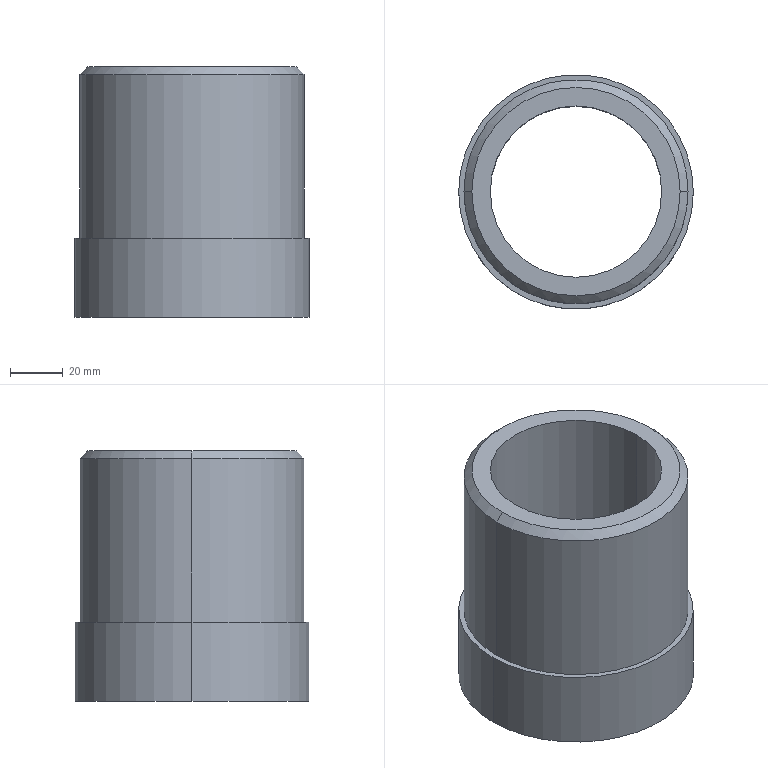Part | SolidWorks | features Chamfer 1, Extrusion 1, ICE 1 | 1 solid | 11 faces | box 89 x 89 x 95 mm | volume 239064 mm3 | cylinder 6 | plane 3 | cone 2 | commonest cylinder face diameters 65 x2 85 x2 89 x2
STEP:
#1=CARTESIAN_POINT('',(39.5,0.,95.));
#2=VERTEX_POINT('',#1);
#3=CARTESIAN_POINT('',(-39.5,0.,95.));
#4=VERTEX_POINT('',#3);
#5=CARTESIAN_POINT('',(0.,0.,95.));
#6=DIRECTION('',(0.,0.,1.));
#7=DIRECTION('',(1.,0.,0.));
#8=AXIS2_PLACEMENT_3D('',#5,#6,#7);
#9=CIRCLE('',#8,39.5);
#10=EDGE_CURVE('',#2,#4,#9,.T.);
#11=ORIENTED_EDGE('',*,*,#10,.F.);
#12=CARTESIAN_POINT('',(42.5,0.,92.));
#13=VERTEX_POINT('',#12);
#14=CARTESIAN_POINT('',(39.5,0.,95.));
#15=DIRECTION('',(0.7071,0.,-0.7071));
#16=VECTOR('',#15,1000.);
#17=LINE('',#14,#16);
#18=EDGE_CURVE('',#2,#13,#17,.T.);
#19=ORIENTED_EDGE('',*,*,#18,.T.);
#20=CARTESIAN_POINT('',(-42.5,0.,92.));
#21=VERTEX_POINT('',#20);
#22=CARTESIAN_POINT('',(0.,0.,92.));
#23=DIRECTION('',(0.,0.,-1.));
#24=DIRECTION('',(1.,0.,0.));
#25=AXIS2_PLACEMENT_3D('',#22,#23,#24);
#26=CIRCLE('',#25,42.5);
#27=EDGE_CURVE('',#21,#13,#26,.T.);
#28=ORIENTED_EDGE('',*,*,#27,.F.);
#29=CARTESIAN_POINT('',(-39.5,0.,95.));
#30=DIRECTION('',(-0.7071,0.,-0.7071));
#31=VECTOR('',#30,1000.);
#32=LINE('',#29,#31);
#33=EDGE_CURVE('',#4,#21,#32,.T.);
#34=ORIENTED_EDGE('',*,*,#33,.F.);
#35=EDGE_LOOP('',(#11,#19,#28,#34));
#36=FACE_OUTER_BOUND('',#35,.T.);
#37=CARTESIAN_POINT('',(0.,0.,95.));
#38=DIRECTION('',(0.,0.,-1.));
#39=DIRECTION('',(-1.,0.,0.));
#40=AXIS2_PLACEMENT_3D('',#37,#38,#39);
#41=CONICAL_SURFACE('',#40,39.5,0.7854);
#42=ADVANCED_FACE('',(#36),#41,.T.);
#43=CARTESIAN_POINT('',(42.5,0.,30.));
#44=VERTEX_POINT('',#43);
#45=CARTESIAN_POINT('',(-42.5,0.,30.));
#46=VERTEX_POINT('',#45);
#47=CARTESIAN_POINT('',(0.,0.,30.));
#48=DIRECTION('',(0.,0.,1.));
#49=DIRECTION('',(1.,0.,0.));
#50=AXIS2_PLACEMENT_3D('',#47,#48,#49);
#51=CIRCLE('',#50,42.5);
#52=EDGE_CURVE('',#44,#46,#51,.T.);
#53=ORIENTED_EDGE('',*,*,#52,.T.);
#54=CARTESIAN_POINT('',(-42.5,0.,30.));
#55=DIRECTION('',(0.,0.,1.));
#56=VECTOR('',#55,1000.);
#57=LINE('',#54,#56);
#58=EDGE_CURVE('',#46,#21,#57,.T.);
#59=ORIENTED_EDGE('',*,*,#58,.T.);
#60=ORIENTED_EDGE('',*,*,#27,.T.);
#61=CARTESIAN_POINT('',(42.5,0.,30.));
#62=DIRECTION('',(0.,0.,1.));
#63=VECTOR('',#62,1000.);
#64=LINE('',#61,#63);
#65=EDGE_CURVE('',#44,#13,#64,.T.);
#66=ORIENTED_EDGE('',*,*,#65,.F.);
#67=EDGE_LOOP('',(#53,#59,#60,#66));
#68=FACE_OUTER_BOUND('',#67,.T.);
#69=CARTESIAN_POINT('',(0.,0.,30.));
#70=DIRECTION('',(0.,0.,1.));
#71=DIRECTION('',(1.,0.,0.));
#72=AXIS2_PLACEMENT_3D('',#69,#70,#71);
#73=CYLINDRICAL_SURFACE('',#72,42.5);
#74=ADVANCED_FACE('',(#68),#73,.T.);
#75=CARTESIAN_POINT('',(-32.5,0.,95.));
#76=VERTEX_POINT('',#75);
#77=CARTESIAN_POINT('',(32.5,0.,95.));
#78=VERTEX_POINT('',#77);
#79=CARTESIAN_POINT('',(0.,0.,95.));
#80=DIRECTION('',(0.,0.,1.));
#81=DIRECTION('',(1.,0.,0.));
#82=AXIS2_PLACEMENT_3D('',#79,#80,#81);
#83=CIRCLE('',#82,32.5);
#84=EDGE_CURVE('',#76,#78,#83,.T.);
#85=ORIENTED_EDGE('',*,*,#84,.T.);
#86=CARTESIAN_POINT('',(32.5,0.,0.));
#87=VERTEX_POINT('',#86);
#88=CARTESIAN_POINT('',(32.5,0.,95.));
#89=DIRECTION('',(0.,0.,-1.));
#90=VECTOR('',#89,1000.);
#91=LINE('',#88,#90);
#92=EDGE_CURVE('',#78,#87,#91,.T.);
#93=ORIENTED_EDGE('',*,*,#92,.T.);
#94=CARTESIAN_POINT('',(-32.5,0.,0.));
#95=VERTEX_POINT('',#94);
#96=CARTESIAN_POINT('',(0.,0.,0.));
#97=DIRECTION('',(0.,0.,1.));
#98=DIRECTION('',(1.,0.,0.));
#99=AXIS2_PLACEMENT_3D('',#96,#97,#98);
#100=CIRCLE('',#99,32.5);
#101=EDGE_CURVE('',#95,#87,#100,.T.);
#102=ORIENTED_EDGE('',*,*,#101,.F.);
#103=CARTESIAN_POINT('',(-32.5,0.,95.));
#104=DIRECTION('',(0.,0.,-1.));
#105=VECTOR('',#104,1000.);
#106=LINE('',#103,#105);
#107=EDGE_CURVE('',#76,#95,#106,.T.);
#108=ORIENTED_EDGE('',*,*,#107,.F.);
#109=EDGE_LOOP('',(#85,#93,#102,#108));
#110=FACE_OUTER_BOUND('',#109,.T.);
#111=CARTESIAN_POINT('',(0.,0.,95.));
#112=DIRECTION('',(0.,0.,-1.));
#113=DIRECTION('',(-1.,0.,0.));
#114=AXIS2_PLACEMENT_3D('',#111,#112,#113);
#115=CYLINDRICAL_SURFACE('',#114,32.5);
#116=ADVANCED_FACE('',(#110),#115,.F.);
#117=CARTESIAN_POINT('',(44.5,0.,30.));
#118=VERTEX_POINT('',#117);
#119=CARTESIAN_POINT('',(-44.5,0.,30.));
#120=VERTEX_POINT('',#119);
#121=CARTESIAN_POINT('',(0.,0.,30.));
#122=DIRECTION('',(0.,0.,1.));
#123=DIRECTION('',(1.,0.,0.));
#124=AXIS2_PLACEMENT_3D('',#121,#122,#123);
#125=CIRCLE('',#124,44.5);
#126=EDGE_CURVE('',#118,#120,#125,.T.);
#127=ORIENTED_EDGE('',*,*,#126,.F.);
#128=CARTESIAN_POINT('',(44.5,0.,0.));
#129=VERTEX_POINT('',#128);
#130=CARTESIAN_POINT('',(44.5,0.,95.));
#131=DIRECTION('',(0.,0.,-1.));
#132=VECTOR('',#131,1000.);
#133=LINE('',#130,#132);
#134=EDGE_CURVE('',#118,#129,#133,.T.);
#135=ORIENTED_EDGE('',*,*,#134,.T.);
#136=CARTESIAN_POINT('',(-44.5,0.,0.));
#137=VERTEX_POINT('',#136);
#138=CARTESIAN_POINT('',(0.,0.,0.));
#139=DIRECTION('',(0.,0.,1.));
#140=DIRECTION('',(1.,0.,0.));
#141=AXIS2_PLACEMENT_3D('',#138,#139,#140);
#142=CIRCLE('',#141,44.5);
#143=EDGE_CURVE('',#129,#137,#142,.T.);
#144=ORIENTED_EDGE('',*,*,#143,.T.);
#145=CARTESIAN_POINT('',(-44.5,0.,95.));
#146=DIRECTION('',(0.,0.,-1.));
#147=VECTOR('',#146,1000.);
#148=LINE('',#145,#147);
#149=EDGE_CURVE('',#120,#137,#148,.T.);
#150=ORIENTED_EDGE('',*,*,#149,.F.);
#151=EDGE_LOOP('',(#127,#135,#144,#150));
#152=FACE_OUTER_BOUND('',#151,.T.);
#153=CARTESIAN_POINT('',(0.,0.,95.));
#154=DIRECTION('',(0.,0.,-1.));
#155=DIRECTION('',(-1.,0.,0.));
#156=AXIS2_PLACEMENT_3D('',#153,#154,#155);
#157=CYLINDRICAL_SURFACE('',#156,44.5);
#158=ADVANCED_FACE('',(#152),#157,.T.);
#159=CARTESIAN_POINT('',(0.,0.,95.));
#160=DIRECTION('',(0.,0.,1.));
#161=DIRECTION('',(1.,0.,0.));
#162=AXIS2_PLACEMENT_3D('',#159,#160,#161);
#163=CIRCLE('',#162,39.5);
#164=EDGE_CURVE('',#4,#2,#163,.T.);
#165=ORIENTED_EDGE('',*,*,#164,.T.);
#166=ORIENTED_EDGE('',*,*,#10,.T.);
#167=EDGE_LOOP('',(#165,#166));
#168=FACE_OUTER_BOUND('',#167,.T.);
#169=ORIENTED_EDGE('',*,*,#84,.F.);
#170=CARTESIAN_POINT('',(0.,0.,95.));
#171=DIRECTION('',(0.,0.,1.));
#172=DIRECTION('',(1.,0.,0.));
#173=AXIS2_PLACEMENT_3D('',#170,#171,#172);
#174=CIRCLE('',#173,32.5);
#175=EDGE_CURVE('',#78,#76,#174,.T.);
#176=ORIENTED_EDGE('',*,*,#175,.F.);
#177=EDGE_LOOP('',(#169,#176));
#178=FACE_BOUND('',#177,.T.);
#179=CARTESIAN_POINT('',(0.,0.,95.));
#180=DIRECTION('',(0.,0.,1.));
#181=DIRECTION('',(1.,0.,0.));
#182=AXIS2_PLACEMENT_3D('',#179,#180,#181);
#183=PLANE('',#182);
#184=ADVANCED_FACE('',(#168,#178),#183,.T.);
#185=ORIENTED_EDGE('',*,*,#134,.F.);
#186=CARTESIAN_POINT('',(0.,0.,30.));
#187=DIRECTION('',(0.,0.,1.));
#188=DIRECTION('',(1.,0.,0.));
#189=AXIS2_PLACEMENT_3D('',#186,#187,#188);
#190=CIRCLE('',#189,44.5);
#191=EDGE_CURVE('',#120,#118,#190,.T.);
#192=ORIENTED_EDGE('',*,*,#191,.F.);
#193=ORIENTED_EDGE('',*,*,#149,.T.);
#194=CARTESIAN_POINT('',(0.,0.,0.));
#195=DIRECTION('',(0.,0.,1.));
#196=DIRECTION('',(1.,0.,0.));
#197=AXIS2_PLACEMENT_3D('',#194,#195,#196);
#198=CIRCLE('',#197,44.5);
#199=EDGE_CURVE('',#137,#129,#198,.T.);
#200=ORIENTED_EDGE('',*,*,#199,.T.);
#201=EDGE_LOOP('',(#185,#192,#193,#200));
#202=FACE_OUTER_BOUND('',#201,.T.);
#203=CARTESIAN_POINT('',(0.,0.,95.));
#204=DIRECTION('',(0.,0.,-1.));
#205=DIRECTION('',(-1.,0.,0.));
#206=AXIS2_PLACEMENT_3D('',#203,#204,#205);
#207=CYLINDRICAL_SURFACE('',#206,44.5);
#208=ADVANCED_FACE('',(#202),#207,.T.);
#209=ORIENTED_EDGE('',*,*,#199,.F.);
#210=ORIENTED_EDGE('',*,*,#143,.F.);
#211=EDGE_LOOP('',(#209,#210));
#212=FACE_OUTER_BOUND('',#211,.T.);
#213=ORIENTED_EDGE('',*,*,#101,.T.);
#214=CARTESIAN_POINT('',(0.,0.,0.));
#215=DIRECTION('',(0.,0.,1.));
#216=DIRECTION('',(1.,0.,0.));
#217=AXIS2_PLACEMENT_3D('',#214,#215,#216);
#218=CIRCLE('',#217,32.5);
#219=EDGE_CURVE('',#87,#95,#218,.T.);
#220=ORIENTED_EDGE('',*,*,#219,.T.);
#221=EDGE_LOOP('',(#213,#220));
#222=FACE_BOUND('',#221,.T.);
#223=CARTESIAN_POINT('',(0.,0.,0.));
#224=DIRECTION('',(0.,0.,1.));
#225=DIRECTION('',(1.,0.,0.));
#226=AXIS2_PLACEMENT_3D('',#223,#224,#225);
#227=PLANE('',#226);
#228=ADVANCED_FACE('',(#212,#222),#227,.F.);
#229=ORIENTED_EDGE('',*,*,#92,.F.);
#230=ORIENTED_EDGE('',*,*,#175,.T.);
#231=ORIENTED_EDGE('',*,*,#107,.T.);
#232=ORIENTED_EDGE('',*,*,#219,.F.);
#233=EDGE_LOOP('',(#229,#230,#231,#232));
#234=FACE_OUTER_BOUND('',#233,.T.);
#235=CARTESIAN_POINT('',(0.,0.,95.));
#236=DIRECTION('',(0.,0.,-1.));
#237=DIRECTION('',(-1.,0.,0.));
#238=AXIS2_PLACEMENT_3D('',#235,#236,#237);
#239=CYLINDRICAL_SURFACE('',#238,32.5);
#240=ADVANCED_FACE('',(#234),#239,.F.);
#241=ORIENTED_EDGE('',*,*,#52,.F.);
#242=CARTESIAN_POINT('',(0.,0.,30.));
#243=DIRECTION('',(0.,0.,1.));
#244=DIRECTION('',(1.,0.,0.));
#245=AXIS2_PLACEMENT_3D('',#242,#243,#244);
#246=CIRCLE('',#245,42.5);
#247=EDGE_CURVE('',#46,#44,#246,.T.);
#248=ORIENTED_EDGE('',*,*,#247,.F.);
#249=EDGE_LOOP('',(#241,#248));
#250=FACE_BOUND('',#249,.T.);
#251=ORIENTED_EDGE('',*,*,#191,.T.);
#252=ORIENTED_EDGE('',*,*,#126,.T.);
#253=EDGE_LOOP('',(#251,#252));
#254=FACE_OUTER_BOUND('',#253,.T.);
#255=CARTESIAN_POINT('',(0.,0.,30.));
#256=DIRECTION('',(0.,0.,1.));
#257=DIRECTION('',(1.,0.,0.));
#258=AXIS2_PLACEMENT_3D('',#255,#256,#257);
#259=PLANE('',#258);
#260=ADVANCED_FACE('',(#250,#254),#259,.T.);
#261=ORIENTED_EDGE('',*,*,#58,.F.);
#262=ORIENTED_EDGE('',*,*,#247,.T.);
#263=ORIENTED_EDGE('',*,*,#65,.T.);
#264=CARTESIAN_POINT('',(0.,0.,92.));
#265=DIRECTION('',(0.,0.,-1.));
#266=DIRECTION('',(1.,0.,0.));
#267=AXIS2_PLACEMENT_3D('',#264,#265,#266);
#268=CIRCLE('',#267,42.5);
#269=EDGE_CURVE('',#13,#21,#268,.T.);
#270=ORIENTED_EDGE('',*,*,#269,.T.);
#271=EDGE_LOOP('',(#261,#262,#263,#270));
#272=FACE_OUTER_BOUND('',#271,.T.);
#273=CARTESIAN_POINT('',(0.,0.,30.));
#274=DIRECTION('',(0.,0.,1.));
#275=DIRECTION('',(1.,0.,0.));
#276=AXIS2_PLACEMENT_3D('',#273,#274,#275);
#277=CYLINDRICAL_SURFACE('',#276,42.5);
#278=ADVANCED_FACE('',(#272),#277,.T.);
#279=ORIENTED_EDGE('',*,*,#18,.F.);
#280=ORIENTED_EDGE('',*,*,#164,.F.);
#281=ORIENTED_EDGE('',*,*,#33,.T.);
#282=ORIENTED_EDGE('',*,*,#269,.F.);
#283=EDGE_LOOP('',(#279,#280,#281,#282));
#284=FACE_OUTER_BOUND('',#283,.T.);
#285=CARTESIAN_POINT('',(0.,0.,95.));
#286=DIRECTION('',(0.,0.,-1.));
#287=DIRECTION('',(-1.,0.,0.));
#288=AXIS2_PLACEMENT_3D('',#285,#286,#287);
#289=CONICAL_SURFACE('',#288,39.5,0.7854);
#290=ADVANCED_FACE('',(#284),#289,.T.);
#291=CLOSED_SHELL('',(#42,#74,#116,#158,#184,#208,#228,#240,#260,#278,#290));
#292=MANIFOLD_SOLID_BREP('',#291);
#293=CARTESIAN_POINT('',(0.,0.,0.));
#294=DIRECTION('',(0.,0.,1.));
#295=DIRECTION('',(1.,0.,0.));
#296=AXIS2_PLACEMENT_3D('',#293,#294,#295);
#297=(LENGTH_UNIT()NAMED_UNIT(*)SI_UNIT(.MILLI.,.METRE.));
#298=UNCERTAINTY_MEASURE_WITH_UNIT(LENGTH_MEASURE(0.00001),#297,'','');
#299=(NAMED_UNIT(*)PLANE_ANGLE_UNIT()SI_UNIT($,.RADIAN.));
#300=(NAMED_UNIT(*)SI_UNIT($,.STERADIAN.)SOLID_ANGLE_UNIT());
#301=(GEOMETRIC_REPRESENTATION_CONTEXT(3)GLOBAL_UNCERTAINTY_ASSIGNED_CONTEXT((#298))GLOBAL_UNIT_ASSIGNED_CONTEXT((#297,#299,#300))REPRESENTATION_CONTEXT('',''));
#302=ADVANCED_BREP_SHAPE_REPRESENTATION('',(#292,#296),#301);